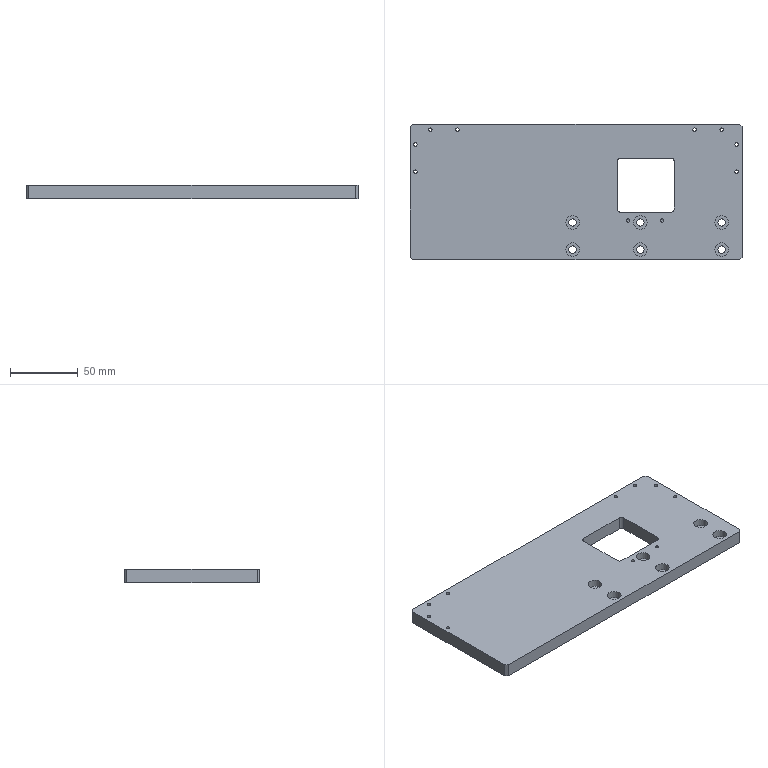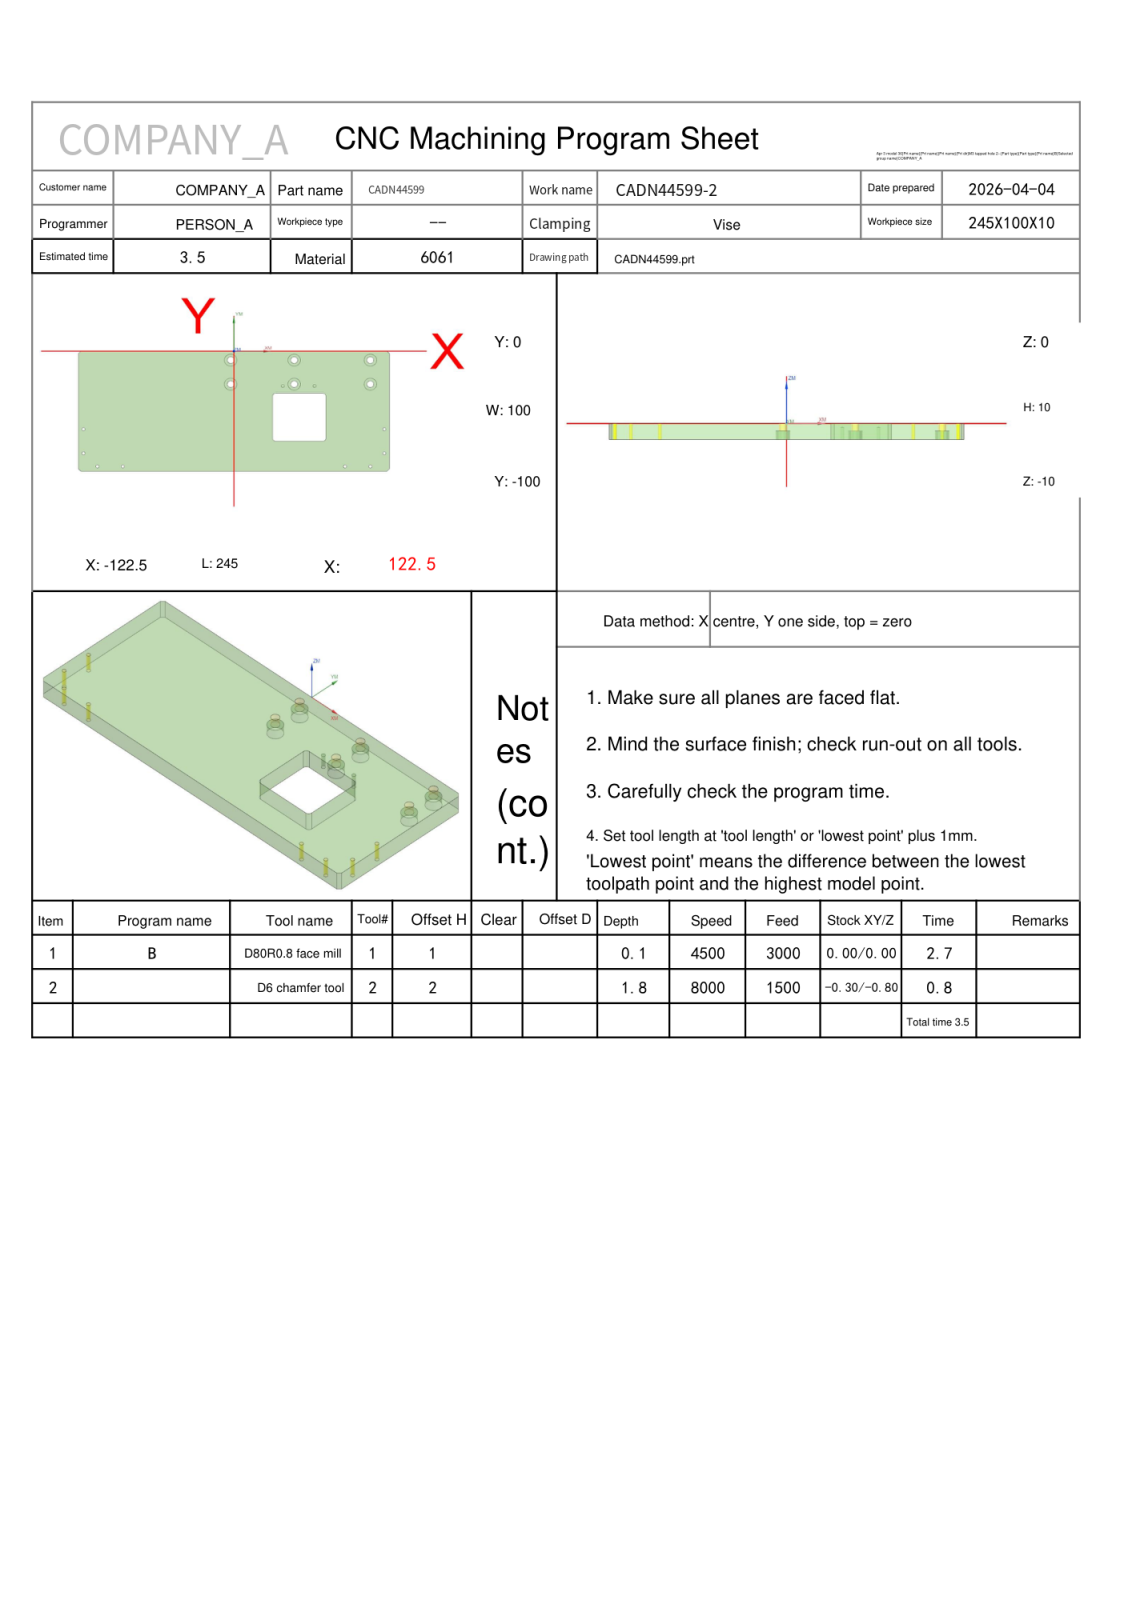NC program | NX | posted by the shop | part box 245 x 100 x 10 mm
Whole program:
%
O0001
(Machine time: 3.87 MIN)
(===Total Tool:2===)
(T1=D80R0.8 face mill D=80.  R=0.8  D-  H01 Z=0.    )
(T2=D6 chamfer tool   D=6.   R=0.   D-  H02 Z=-1.75 )
G80 G90 G17 G49 G40
G91 G28 Z0
M01
N1 T01 M06
(D80R0.8 face mill  D=80. R=0.8 H=01 ce=0.20 di=0.10)
G00 G90 G54 X174.5 Y-95. M03 S4500
G43 H01 Z20.
M08
Z3.525
G01 Z1.525 F3000.
X162.5
X-155.3
G02 X-162.5 Y-87.8 I0.0 J7.2
G01 Y-57.2
G02 X-155.3 Y-50. I7.2 J0.0
G01 X155.3
G03 X162.5 Y-42.8 I0.0 J7.2
G01 Y-12.2
G03 X155.3 Y-5. I-7.2 J0.0
G01 X-162.5
X-174.5
Z3.525
G00 Z5.
X174.5 Y-95.
Z3.05
G01 Z1.05
X162.5
X-155.3
G02 X-162.5 Y-87.8 I0.0 J7.2
G01 Y-57.2
G02 X-155.3 Y-50. I7.2 J0.0
G01 X155.3
G03 X162.5 Y-42.8 I0.0 J7.2
G01 Y-12.2
G03 X155.3 Y-5. I-7.2 J0.0
G01 X-162.5
X-174.5
Z3.05
G00 Z4.525
X174.5 Y-95.
Z2.575
G01 Z.575
X162.5
X-155.3
G02 X-162.5 Y-87.8 I0.0 J7.2
G01 Y-57.2
G02 X-155.3 Y-50. I7.2 J0.0
G01 X155.3
G03 X162.5 Y-42.8 I0.0 J7.2
G01 Y-12.2
G03 X155.3 Y-5. I-7.2 J0.0
G01 X-162.5
X-174.5
Z2.575
G00 Z4.05
X174.5 Y-95.
Z2.1
G01 Z.1
X162.5
X-155.3
G02 X-162.5 Y-87.8 I0.0 J7.2
G01 Y-57.2
G02 X-155.3 Y-50. I7.2 J0.0
G01 X155.3
G03 X162.5 Y-42.8 I0.0 J7.2
G01 Y-12.2
G03 X155.3 Y-5. I-7.2 J0.0
G01 X-162.5
X-174.5
Z2.1
G00 Z20.
G00 G90 X174.5 Y-95. M03 S4500
Z20.
Z2.
G01 Z0.0 F1000.
X162.5
X-162.5
Y-50.
X162.5
Y-5.
X-162.5
X-174.5
Z2.
G00 Z20.
G91 G28 Z0.0
M05
M09
G91 G28 Z0.0
M01
N2 T02 M06
(D6 chamfer tool  D=6. R=0. H=02 ce=0.00 di=0.00)
G00 G90 G54 X118.5 Y-65. M03 S8000
G43 H02 Z20.
M08
G98 G81 X118.5 Y-65. Z-1.75 R3. F1000.
Y-85.
X107.5 Y-96.
X87.5
X-87.5
X-107.5
X-118.5 Y-85.
Y-65.
G80
G00 Z20.
G00 G90 X-2.565 Y-26.853 M03 S8000
Z20.
Z-.9
G01 Z-1.4 F1200.
X-2.65 Y-26.
G03 X-4.15 Y-27.5 I0.0 J-1.5
X-2.5 Y-29.15 I1.65 J0.0
X-.85 Y-27.5 I0.0 J1.65
X-2.5 Y-25.85 I-1.65 J0.0
X-4.15 Y-27.5 I0.0 J-1.65
X-2.65 Y-29. I1.5 J0.0
G01 X-2.565 Y-28.147
Z-.9
G00 Z20.
Y-6.853
Z-.9
G01 Z-1.4
X-2.65 Y-6.
G03 X-4.15 Y-7.5 I0.0 J-1.5
X-2.5 Y-9.15 I1.65 J0.0
X-.85 Y-7.5 I0.0 J1.65
X-2.5 Y-5.85 I-1.65 J0.0
X-4.15 Y-7.5 I0.0 J-1.65
X-2.65 Y-9. I1.5 J0.0
G01 X-2.565 Y-8.147
Z-.9
G00 Z20.
X47.435 Y-6.853
Z-.9
G01 Z-1.4
X47.35 Y-6.
G03 X45.85 Y-7.5 I0.0 J-1.5
X47.5 Y-9.15 I1.65 J0.0
X49.15 Y-7.5 I0.0 J1.65
X47.5 Y-5.85 I-1.65 J0.0
X45.85 Y-7.5 I0.0 J-1.65
X47.35 Y-9. I1.5 J0.0
G01 X47.435 Y-8.147
Z-.9
G00 Z20.
Y-26.853
Z-.9
G01 Z-1.4
X47.35 Y-26.
G03 X45.85 Y-27.5 I0.0 J-1.5
X47.5 Y-29.15 I1.65 J0.0
X49.15 Y-27.5 I0.0 J1.65
X47.5 Y-25.85 I-1.65 J0.0
X45.85 Y-27.5 I0.0 J-1.65
X47.35 Y-29. I1.5 J0.0
G01 X47.435 Y-28.147
Z-.9
G00 Z20.
X107.435 Y-26.853
Z-.9
G01 Z-1.4
X107.35 Y-26.
G03 X105.85 Y-27.5 I0.0 J-1.5
X107.5 Y-29.15 I1.65 J0.0
X109.15 Y-27.5 I0.0 J1.65
X107.5 Y-25.85 I-1.65 J0.0
X105.85 Y-27.5 I0.0 J-1.65
X107.35 Y-29. I1.5 J0.0
G01 X107.435 Y-28.147
Z-.9
G00 Z20.
Y-6.853
Z-.9
G01 Z-1.4
X107.35 Y-6.
G03 X105.85 Y-7.5 I0.0 J-1.5
X107.5 Y-9.15 I1.65 J0.0
X109.15 Y-7.5 I0.0 J1.65
X107.5 Y-5.85 I-1.65 J0.0
X105.85 Y-7.5 I0.0 J-1.65
X107.35 Y-9. I1.5 J0.0
G01 X107.435 Y-8.147
Z-.9
G00 Z20.
G00 G90 X-111.546 Y-100.7 M03 S7000
Z20.
Z2.5
G01 X-120.376 Z-.714 F1500.
X-120.453 Z-.742
X-120.66 Y-100.662 Z-.819
X-120.855 Y-100.581 Z-.895
X-121.028 Y-100.462 Z-.972
X-121.083 Y-100.407 Z-1.
X-122.907 Y-98.583
G02 X-123.2 Y-97.876 I.707 J.707
G01 Y-2.124
G02 X-122.907 Y-1.417 I1. J0.0
G01 X-121.083 Y.407
G02 X-120.376 Y.7 I.707 J-.707
G01 X120.376
G02 X121.083 Y.407 I0.0 J-1.
G01 X122.907 Y-1.417
G02 X123.2 Y-2.124 I-.707 J-.707
G01 Y-97.876
G02 X122.907 Y-98.583 I-1. J0.0
G01 X121.083 Y-100.407
G02 X120.376 Y-100.7 I-.707 J.707
G01 X-120.376
G02 X-121.083 Y-100.407 I0.0 J1.
G01 X-121.436 Y-100.054
Z1.5
G00 Z20.
X39.824 Y-35.7
Z2.5
G01 X32.833 Z-.044
X32.556 Y-35.739 Z-.146
X32.288 Y-35.822 Z-.248
X32.037 Y-35.947 Z-.35
X31.809 Y-36.111 Z-.453
X31.611 Y-36.309 Z-.555
X31.447 Y-36.537 Z-.657
X31.322 Y-36.788 Z-.759
X31.239 Y-37.056 Z-.861
X31.2 Y-37.333 Z-.963
Y-37.435 Z-1.
Y-72.565
G03 X32.935 Y-74.3 I1.735 J0.0
G01 X70.065
G03 X71.8 Y-72.565 I0.0 J1.735
G01 Y-37.435
G03 X70.065 Y-35.7 I-1.735 J0.0
G01 X32.935
G03 X31.2 Y-37.435 I0.0 J-1.735
G01 Y-37.935
Z1.5
G00 Z20.
M05
M09
G91 G28 Z0.0
G91 G28 Y0.0
M30
%